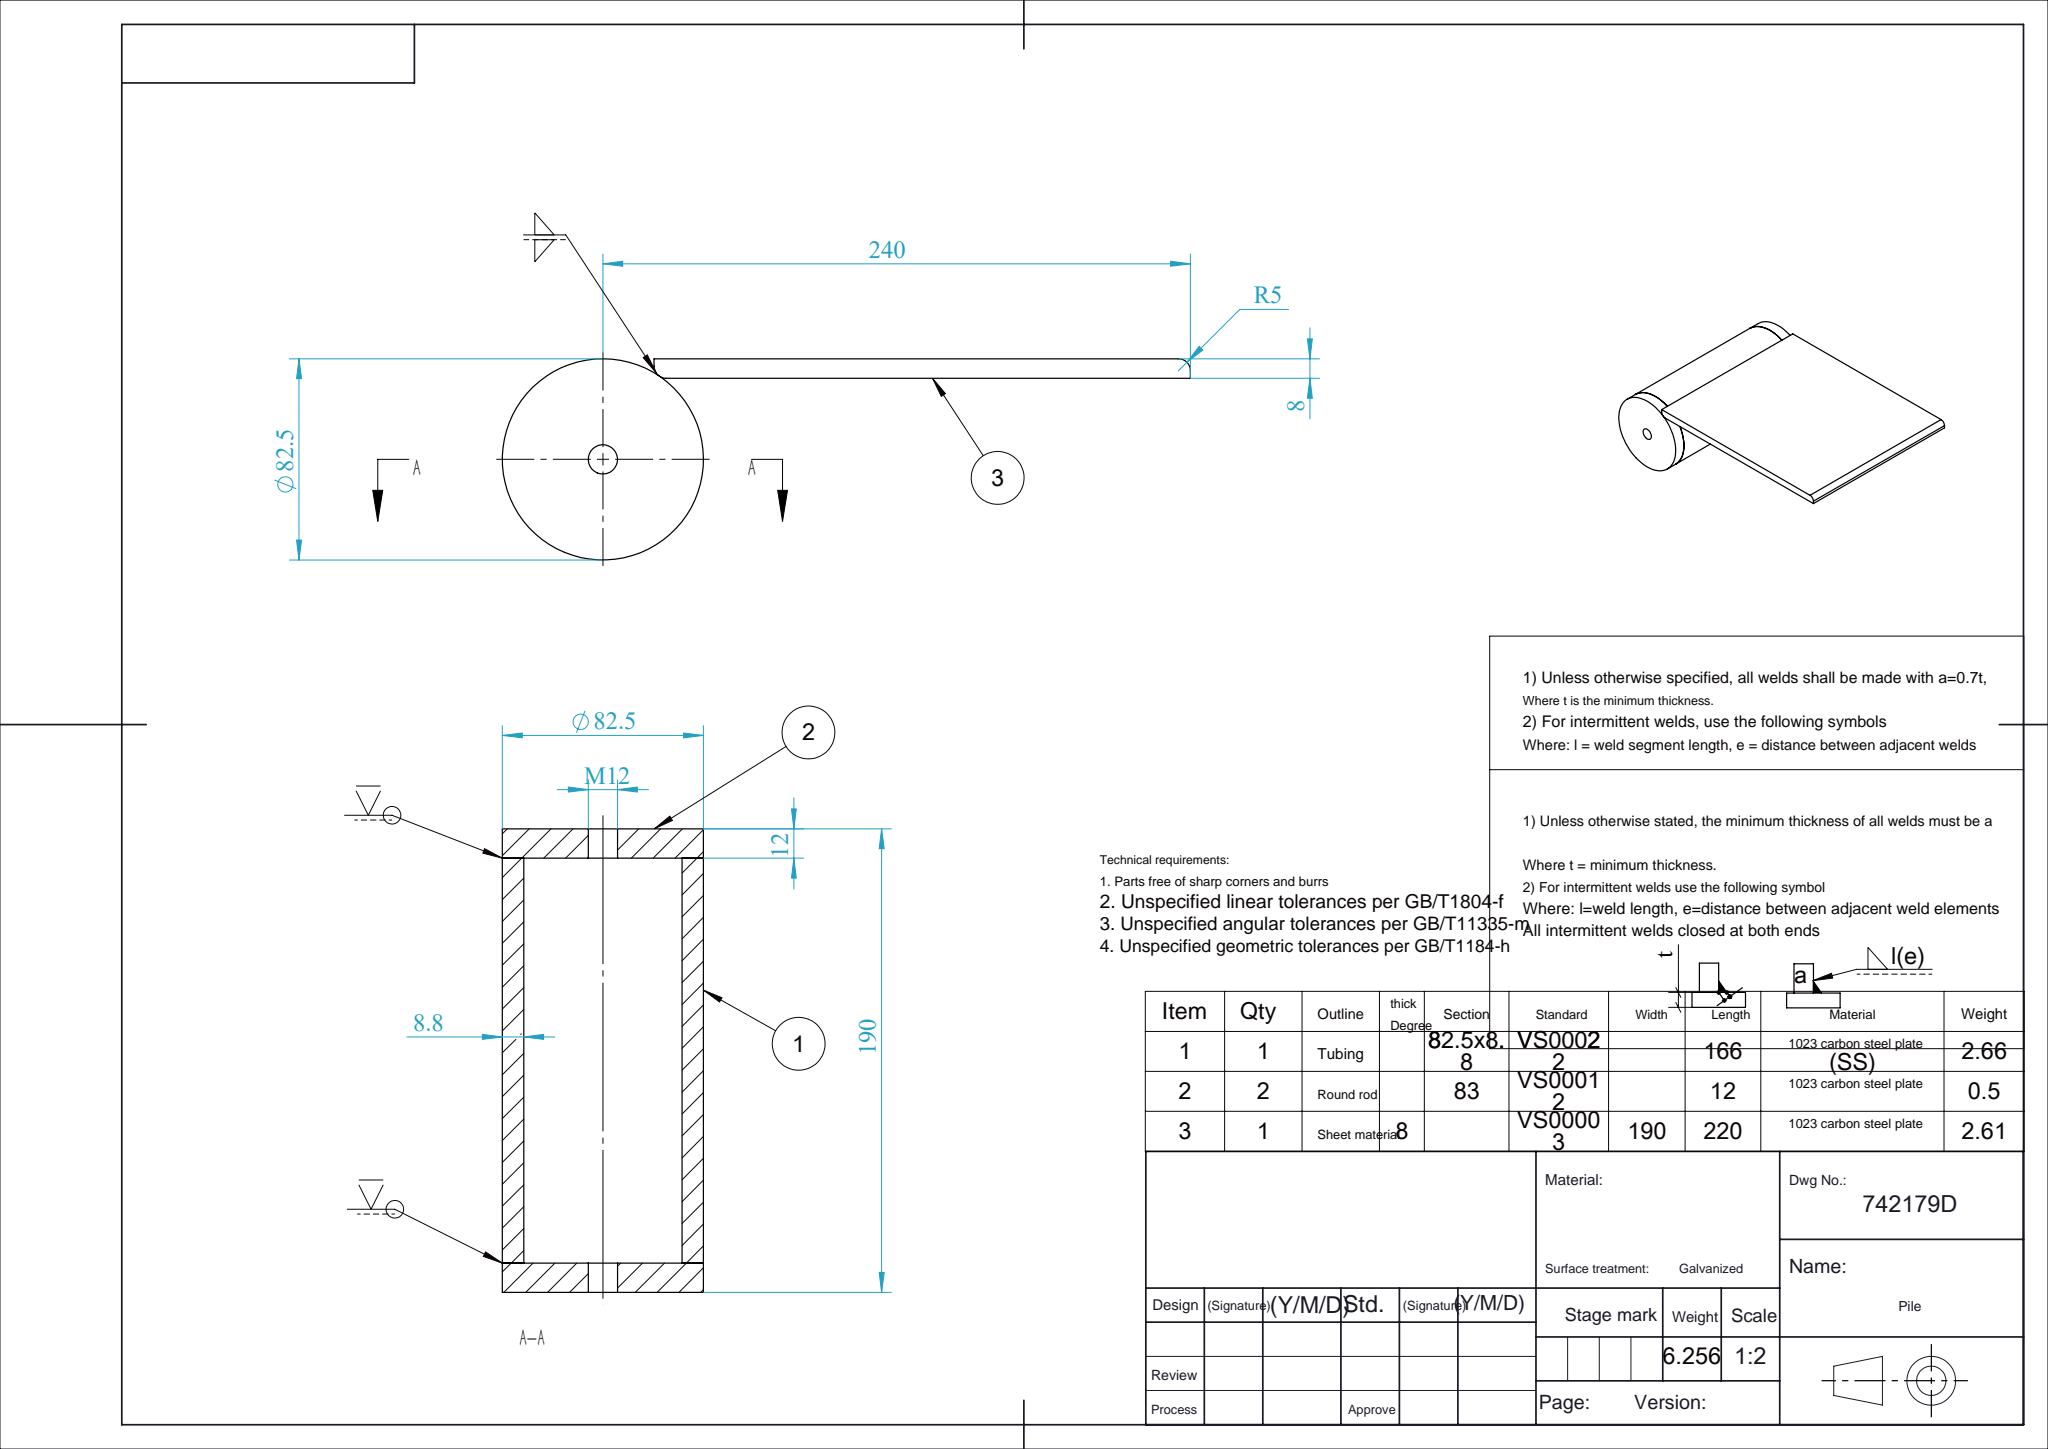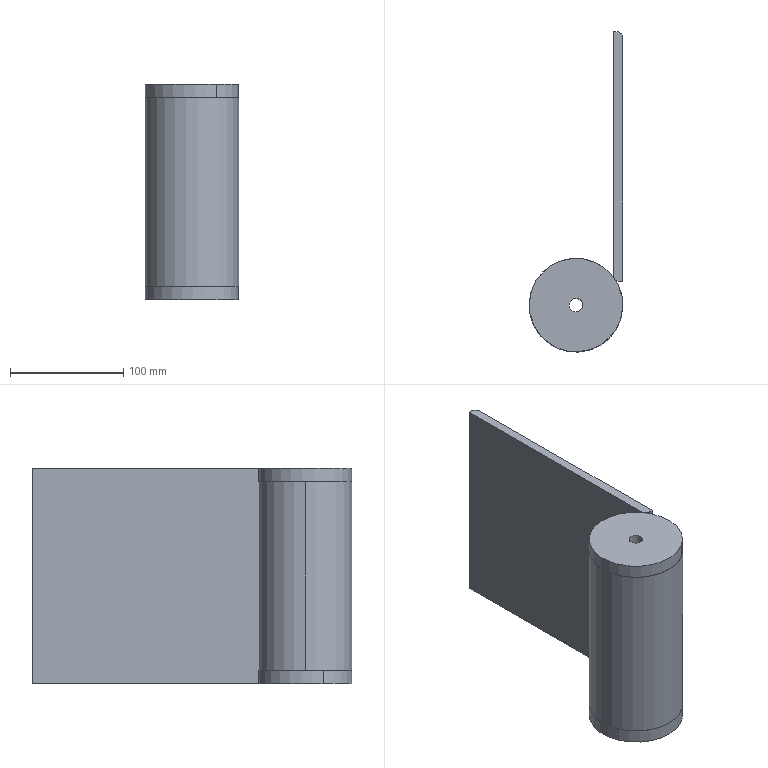Part | SolidWorks | 4 solids | 26 faces | box 82.5 x 282.25 x 190 mm | volume 796169 mm3 | cylinder 14 | plane 12 | commonest cylinder face diameters 82.5 x6 12 x4 10 x2 64.9 x2